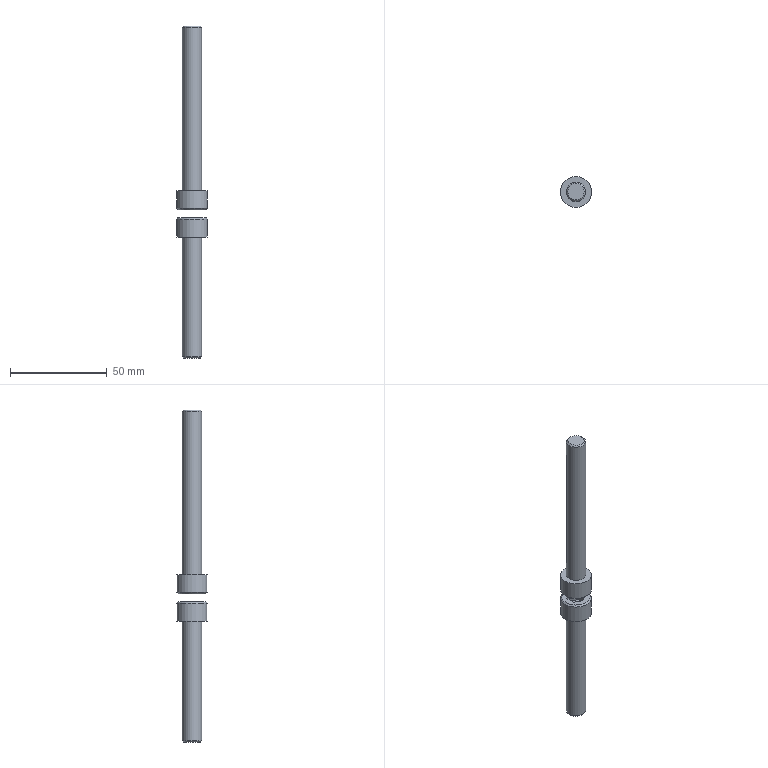Part | STEP file | M10.00-85 | 2 solids | 28 faces | box 16 x 16 x 171.5 mm | volume 14936 mm3 | plane 20 | cylinder 4 | cone 4 | commonest cylinder face diameters 10 x2 16 x2